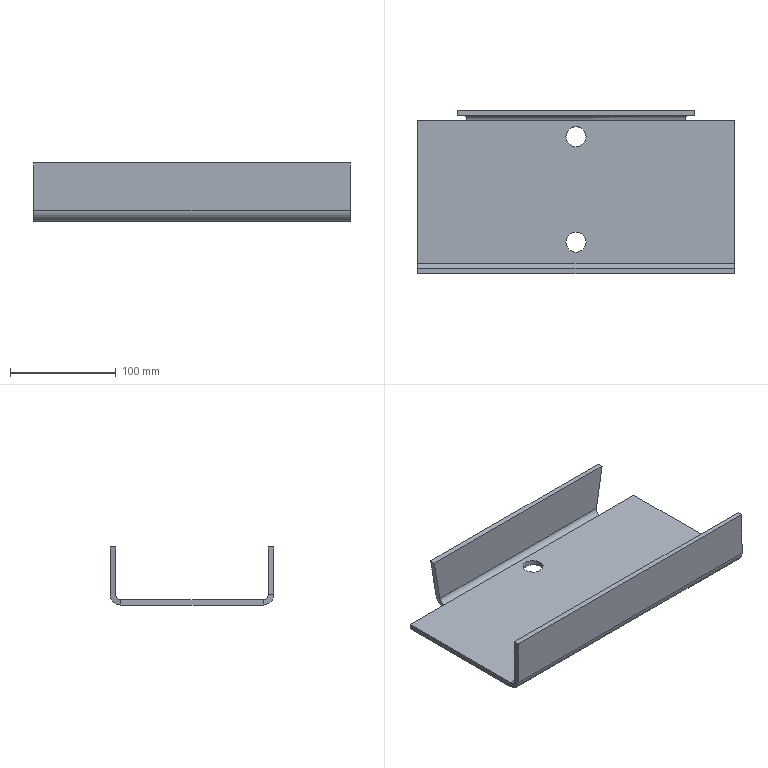Part | SolidWorks | features Split 2, FlatPattern 1, HoleWzd 1, SM3dBend 1, SMBaseFlange 1, SheetMetal 1 | 1 solid | 26 faces | box 300 x 155 x 54.999 mm | volume 345967 mm3 | plane 18 | cylinder 8 | commonest cylinder face diameters 19 x4 10 x2 20 x2
STEP:
#1=CARTESIAN_POINT('',(9.5,52.5,0.));
#2=VERTEX_POINT('',#1);
#3=CARTESIAN_POINT('',(-9.5,52.5,0.));
#4=VERTEX_POINT('',#3);
#5=CARTESIAN_POINT('',(0.,52.5,0.));
#6=DIRECTION('',(0.,0.,-1.));
#7=DIRECTION('',(1.,0.,0.));
#8=AXIS2_PLACEMENT_3D('',#5,#6,#7);
#9=CIRCLE('',#8,9.5);
#10=EDGE_CURVE('',#2,#4,#9,.T.);
#11=ORIENTED_EDGE('',*,*,#10,.F.);
#12=CARTESIAN_POINT('',(9.5,52.5,-5.));
#13=VERTEX_POINT('',#12);
#14=CARTESIAN_POINT('',(9.5,52.5,-5.));
#15=DIRECTION('',(0.,0.,-1.));
#16=VECTOR('',#15,1000.);
#17=LINE('',#14,#16);
#18=EDGE_CURVE('',#2,#13,#17,.T.);
#19=ORIENTED_EDGE('',*,*,#18,.T.);
#20=CARTESIAN_POINT('',(-9.5,52.5,-5.));
#21=VERTEX_POINT('',#20);
#22=CARTESIAN_POINT('',(0.,52.5,-5.));
#23=DIRECTION('',(0.,0.,-1.));
#24=DIRECTION('',(-1.,0.,0.));
#25=AXIS2_PLACEMENT_3D('',#22,#23,#24);
#26=CIRCLE('',#25,9.5);
#27=EDGE_CURVE('',#13,#21,#26,.T.);
#28=ORIENTED_EDGE('',*,*,#27,.T.);
#29=CARTESIAN_POINT('',(-9.5,52.5,-5.));
#30=DIRECTION('',(0.,0.,-1.));
#31=VECTOR('',#30,1000.);
#32=LINE('',#29,#31);
#33=EDGE_CURVE('',#4,#21,#32,.T.);
#34=ORIENTED_EDGE('',*,*,#33,.F.);
#35=EDGE_LOOP('',(#11,#19,#28,#34));
#36=FACE_OUTER_BOUND('',#35,.T.);
#37=CARTESIAN_POINT('',(0.,52.5,-5.));
#38=DIRECTION('',(0.,0.,-1.));
#39=DIRECTION('',(-1.,0.,0.));
#40=AXIS2_PLACEMENT_3D('',#37,#38,#39);
#41=CYLINDRICAL_SURFACE('',#40,9.5);
#42=ADVANCED_FACE('',(#36),#41,.F.);
#43=CARTESIAN_POINT('',(9.5,-47.5,0.));
#44=VERTEX_POINT('',#43);
#45=CARTESIAN_POINT('',(-9.5,-47.5,0.));
#46=VERTEX_POINT('',#45);
#47=CARTESIAN_POINT('',(0.,-47.5,0.));
#48=DIRECTION('',(0.,0.,-1.));
#49=DIRECTION('',(1.,0.,0.));
#50=AXIS2_PLACEMENT_3D('',#47,#48,#49);
#51=CIRCLE('',#50,9.5);
#52=EDGE_CURVE('',#44,#46,#51,.T.);
#53=ORIENTED_EDGE('',*,*,#52,.F.);
#54=CARTESIAN_POINT('',(9.5,-47.5,-5.));
#55=VERTEX_POINT('',#54);
#56=CARTESIAN_POINT('',(9.5,-47.5,-5.));
#57=DIRECTION('',(0.,0.,-1.));
#58=VECTOR('',#57,1000.);
#59=LINE('',#56,#58);
#60=EDGE_CURVE('',#44,#55,#59,.T.);
#61=ORIENTED_EDGE('',*,*,#60,.T.);
#62=CARTESIAN_POINT('',(-9.5,-47.5,-5.));
#63=VERTEX_POINT('',#62);
#64=CARTESIAN_POINT('',(0.,-47.5,-5.));
#65=DIRECTION('',(0.,0.,-1.));
#66=DIRECTION('',(-1.,0.,0.));
#67=AXIS2_PLACEMENT_3D('',#64,#65,#66);
#68=CIRCLE('',#67,9.5);
#69=EDGE_CURVE('',#55,#63,#68,.T.);
#70=ORIENTED_EDGE('',*,*,#69,.T.);
#71=CARTESIAN_POINT('',(-9.5,-47.5,-5.));
#72=DIRECTION('',(0.,0.,-1.));
#73=VECTOR('',#72,1000.);
#74=LINE('',#71,#73);
#75=EDGE_CURVE('',#46,#63,#74,.T.);
#76=ORIENTED_EDGE('',*,*,#75,.F.);
#77=EDGE_LOOP('',(#53,#61,#70,#76));
#78=FACE_OUTER_BOUND('',#77,.T.);
#79=CARTESIAN_POINT('',(0.,-47.5,-5.));
#80=DIRECTION('',(0.,0.,-1.));
#81=DIRECTION('',(-1.,0.,0.));
#82=AXIS2_PLACEMENT_3D('',#79,#80,#81);
#83=CYLINDRICAL_SURFACE('',#82,9.5);
#84=ADVANCED_FACE('',(#78),#83,.F.);
#85=CARTESIAN_POINT('',(103.165,67.5,-5.));
#86=VERTEX_POINT('',#85);
#87=CARTESIAN_POINT('',(104.001,67.5,0.));
#88=VERTEX_POINT('',#87);
#89=CARTESIAN_POINT('',(101.168,67.5,-16.93));
#90=DIRECTION('',(0.165,0.,0.9863));
#91=VECTOR('',#90,1000.);
#92=LINE('',#89,#91);
#93=EDGE_CURVE('',#86,#88,#92,.T.);
#94=ORIENTED_EDGE('',*,*,#93,.F.);
#95=CARTESIAN_POINT('',(104.838,77.5,5.));
#96=VERTEX_POINT('',#95);
#97=CARTESIAN_POINT('',(103.165,67.5,-5.));
#98=CARTESIAN_POINT('',(103.165,73.358,-5.));
#99=CARTESIAN_POINT('',(103.858,77.5,-0.8579));
#100=CARTESIAN_POINT('',(104.838,77.5,5.));
#101=(BOUNDED_CURVE()B_SPLINE_CURVE(3,(#97,#98,#99,#100),.UNSPECIFIED.,.F.,.F.)B_SPLINE_CURVE_WITH_KNOTS((4,4),(3.142,4.712),.UNSPECIFIED.)CURVE()GEOMETRIC_REPRESENTATION_ITEM()RATIONAL_B_SPLINE_CURVE((1.,0.8047,0.8047,1.))REPRESENTATION_ITEM(''));
#102=EDGE_CURVE('',#86,#96,#101,.T.);
#103=ORIENTED_EDGE('',*,*,#102,.T.);
#104=CARTESIAN_POINT('',(112.368,77.5,49.999));
#105=VERTEX_POINT('',#104);
#106=CARTESIAN_POINT('',(89.077,77.5,-89.187));
#107=DIRECTION('',(-0.165,0.,-0.9863));
#108=VECTOR('',#107,1000.);
#109=LINE('',#106,#108);
#110=EDGE_CURVE('',#105,#96,#109,.T.);
#111=ORIENTED_EDGE('',*,*,#110,.F.);
#112=CARTESIAN_POINT('',(112.368,72.5,49.999));
#113=VERTEX_POINT('',#112);
#114=CARTESIAN_POINT('',(112.368,77.5,49.999));
#115=DIRECTION('',(0.,-1.,0.));
#116=VECTOR('',#115,1000.);
#117=LINE('',#114,#116);
#118=EDGE_CURVE('',#105,#113,#117,.T.);
#119=ORIENTED_EDGE('',*,*,#118,.T.);
#120=CARTESIAN_POINT('',(104.838,72.5,5.));
#121=VERTEX_POINT('',#120);
#122=CARTESIAN_POINT('',(89.077,72.5,-89.187));
#123=DIRECTION('',(-0.165,0.,-0.9863));
#124=VECTOR('',#123,1000.);
#125=LINE('',#122,#124);
#126=EDGE_CURVE('',#113,#121,#125,.T.);
#127=ORIENTED_EDGE('',*,*,#126,.T.);
#128=CARTESIAN_POINT('',(104.001,67.5,0.));
#129=CARTESIAN_POINT('',(104.001,70.429,0.));
#130=CARTESIAN_POINT('',(104.348,72.5,2.071));
#131=CARTESIAN_POINT('',(104.838,72.5,5.));
#132=(BOUNDED_CURVE()B_SPLINE_CURVE(3,(#128,#129,#130,#131),.UNSPECIFIED.,.F.,.F.)B_SPLINE_CURVE_WITH_KNOTS((4,4),(3.142,4.712),.UNSPECIFIED.)CURVE()GEOMETRIC_REPRESENTATION_ITEM()RATIONAL_B_SPLINE_CURVE((1.,0.8047,0.8047,1.))REPRESENTATION_ITEM(''));
#133=EDGE_CURVE('',#88,#121,#132,.T.);
#134=ORIENTED_EDGE('',*,*,#133,.F.);
#135=EDGE_LOOP('',(#94,#103,#111,#119,#127,#134));
#136=FACE_OUTER_BOUND('',#135,.T.);
#137=CARTESIAN_POINT('',(101.168,0.,-16.93));
#138=DIRECTION('',(-0.9863,0.,0.165));
#139=DIRECTION('',(0.165,0.,0.9863));
#140=AXIS2_PLACEMENT_3D('',#137,#138,#139);
#141=PLANE('',#140);
#142=ADVANCED_FACE('',(#136),#141,.F.);
#143=CARTESIAN_POINT('',(-104.032,67.5,0.));
#144=VERTEX_POINT('',#143);
#145=CARTESIAN_POINT('',(-150.,67.5,0.));
#146=VERTEX_POINT('',#145);
#147=CARTESIAN_POINT('',(0.,67.5,0.));
#148=DIRECTION('',(-1.,0.,0.));
#149=VECTOR('',#148,1000.);
#150=LINE('',#147,#149);
#151=EDGE_CURVE('',#144,#146,#150,.T.);
#152=ORIENTED_EDGE('',*,*,#151,.F.);
#153=CARTESIAN_POINT('',(-103.195,67.5,-5.));
#154=VERTEX_POINT('',#153);
#155=CARTESIAN_POINT('',(-101.198,67.5,-16.935));
#156=DIRECTION('',(0.165,0.,-0.9863));
#157=VECTOR('',#156,1000.);
#158=LINE('',#155,#157);
#159=EDGE_CURVE('',#144,#154,#158,.T.);
#160=ORIENTED_EDGE('',*,*,#159,.T.);
#161=CARTESIAN_POINT('',(-150.,67.5,-5.));
#162=VERTEX_POINT('',#161);
#163=CARTESIAN_POINT('',(0.,67.5,-5.));
#164=DIRECTION('',(-1.,0.,0.));
#165=VECTOR('',#164,1000.);
#166=LINE('',#163,#165);
#167=EDGE_CURVE('',#154,#162,#166,.T.);
#168=ORIENTED_EDGE('',*,*,#167,.T.);
#169=CARTESIAN_POINT('',(-150.,67.5,-5.));
#170=DIRECTION('',(0.,0.,-1.));
#171=VECTOR('',#170,1000.);
#172=LINE('',#169,#171);
#173=EDGE_CURVE('',#146,#162,#172,.T.);
#174=ORIENTED_EDGE('',*,*,#173,.F.);
#175=EDGE_LOOP('',(#152,#160,#168,#174));
#176=FACE_OUTER_BOUND('',#175,.T.);
#177=CARTESIAN_POINT('',(0.,67.5,0.));
#178=DIRECTION('',(0.,1.,0.));
#179=DIRECTION('',(0.,0.,1.));
#180=AXIS2_PLACEMENT_3D('',#177,#178,#179);
#181=PLANE('',#180);
#182=ADVANCED_FACE('',(#176),#181,.T.);
#183=CARTESIAN_POINT('',(-150.,-72.5,49.999));
#184=VERTEX_POINT('',#183);
#185=CARTESIAN_POINT('',(150.,-72.5,49.999));
#186=VERTEX_POINT('',#185);
#187=CARTESIAN_POINT('',(-150.,-72.5,49.999));
#188=DIRECTION('',(1.,0.,0.));
#189=VECTOR('',#188,1000.);
#190=LINE('',#187,#189);
#191=EDGE_CURVE('',#184,#186,#190,.T.);
#192=ORIENTED_EDGE('',*,*,#191,.T.);
#193=CARTESIAN_POINT('',(150.,-72.5,5.));
#194=VERTEX_POINT('',#193);
#195=CARTESIAN_POINT('',(150.,-72.5,-198.561));
#196=DIRECTION('',(0.,0.,-1.));
#197=VECTOR('',#196,1000.);
#198=LINE('',#195,#197);
#199=EDGE_CURVE('',#186,#194,#198,.T.);
#200=ORIENTED_EDGE('',*,*,#199,.T.);
#201=CARTESIAN_POINT('',(-150.,-72.5,5.));
#202=VERTEX_POINT('',#201);
#203=CARTESIAN_POINT('',(0.,-72.5,5.));
#204=DIRECTION('',(-1.,0.,0.));
#205=VECTOR('',#204,1000.);
#206=LINE('',#203,#205);
#207=EDGE_CURVE('',#194,#202,#206,.T.);
#208=ORIENTED_EDGE('',*,*,#207,.T.);
#209=CARTESIAN_POINT('',(-150.,-72.5,-198.561));
#210=DIRECTION('',(0.,0.,1.));
#211=VECTOR('',#210,1000.);
#212=LINE('',#209,#211);
#213=EDGE_CURVE('',#202,#184,#212,.T.);
#214=ORIENTED_EDGE('',*,*,#213,.T.);
#215=EDGE_LOOP('',(#192,#200,#208,#214));
#216=FACE_OUTER_BOUND('',#215,.T.);
#217=CARTESIAN_POINT('',(0.,-72.5,-74.281));
#218=DIRECTION('',(0.,1.,0.));
#219=DIRECTION('',(1.,0.,0.));
#220=AXIS2_PLACEMENT_3D('',#217,#218,#219);
#221=PLANE('',#220);
#222=ADVANCED_FACE('',(#216),#221,.T.);
#223=ORIENTED_EDGE('',*,*,#207,.F.);
#224=CARTESIAN_POINT('',(150.,-67.5,0.));
#225=VERTEX_POINT('',#224);
#226=CARTESIAN_POINT('',(150.,-67.5,5.));
#227=DIRECTION('',(-1.,0.,0.));
#228=DIRECTION('',(0.,0.,1.));
#229=AXIS2_PLACEMENT_3D('',#226,#227,#228);
#230=CIRCLE('',#229,5.);
#231=EDGE_CURVE('',#225,#194,#230,.T.);
#232=ORIENTED_EDGE('',*,*,#231,.F.);
#233=CARTESIAN_POINT('',(-150.,-67.5,0.));
#234=VERTEX_POINT('',#233);
#235=CARTESIAN_POINT('',(0.,-67.5,0.));
#236=DIRECTION('',(-1.,0.,0.));
#237=VECTOR('',#236,1000.);
#238=LINE('',#235,#237);
#239=EDGE_CURVE('',#225,#234,#238,.T.);
#240=ORIENTED_EDGE('',*,*,#239,.T.);
#241=CARTESIAN_POINT('',(-150.,-67.5,5.));
#242=DIRECTION('',(1.,0.,0.));
#243=DIRECTION('',(0.,0.,1.));
#244=AXIS2_PLACEMENT_3D('',#241,#242,#243);
#245=CIRCLE('',#244,5.);
#246=EDGE_CURVE('',#202,#234,#245,.T.);
#247=ORIENTED_EDGE('',*,*,#246,.F.);
#248=EDGE_LOOP('',(#223,#232,#240,#247));
#249=FACE_OUTER_BOUND('',#248,.T.);
#250=CARTESIAN_POINT('',(300.273,-67.5,5.));
#251=DIRECTION('',(-1.,0.,0.));
#252=DIRECTION('',(0.,0.,1.));
#253=AXIS2_PLACEMENT_3D('',#250,#251,#252);
#254=CYLINDRICAL_SURFACE('',#253,5.);
#255=ADVANCED_FACE('',(#249),#254,.F.);
#256=CARTESIAN_POINT('',(150.,-77.5,5.));
#257=VERTEX_POINT('',#256);
#258=CARTESIAN_POINT('',(-150.,-77.5,5.));
#259=VERTEX_POINT('',#258);
#260=CARTESIAN_POINT('',(0.,-77.5,5.));
#261=DIRECTION('',(-1.,0.,0.));
#262=VECTOR('',#261,1000.);
#263=LINE('',#260,#262);
#264=EDGE_CURVE('',#257,#259,#263,.T.);
#265=ORIENTED_EDGE('',*,*,#264,.F.);
#266=CARTESIAN_POINT('',(150.,-77.5,49.999));
#267=VERTEX_POINT('',#266);
#268=CARTESIAN_POINT('',(150.,-77.5,-198.561));
#269=DIRECTION('',(0.,0.,-1.));
#270=VECTOR('',#269,1000.);
#271=LINE('',#268,#270);
#272=EDGE_CURVE('',#267,#257,#271,.T.);
#273=ORIENTED_EDGE('',*,*,#272,.F.);
#274=CARTESIAN_POINT('',(-150.,-77.5,49.999));
#275=VERTEX_POINT('',#274);
#276=CARTESIAN_POINT('',(-150.,-77.5,49.999));
#277=DIRECTION('',(1.,0.,0.));
#278=VECTOR('',#277,1000.);
#279=LINE('',#276,#278);
#280=EDGE_CURVE('',#275,#267,#279,.T.);
#281=ORIENTED_EDGE('',*,*,#280,.F.);
#282=CARTESIAN_POINT('',(-150.,-77.5,-198.561));
#283=DIRECTION('',(0.,0.,1.));
#284=VECTOR('',#283,1000.);
#285=LINE('',#282,#284);
#286=EDGE_CURVE('',#259,#275,#285,.T.);
#287=ORIENTED_EDGE('',*,*,#286,.F.);
#288=EDGE_LOOP('',(#265,#273,#281,#287));
#289=FACE_OUTER_BOUND('',#288,.T.);
#290=CARTESIAN_POINT('',(0.,-77.5,-74.281));
#291=DIRECTION('',(0.,1.,0.));
#292=DIRECTION('',(1.,0.,0.));
#293=AXIS2_PLACEMENT_3D('',#290,#291,#292);
#294=PLANE('',#293);
#295=ADVANCED_FACE('',(#289),#294,.F.);
#296=CARTESIAN_POINT('',(150.,-67.5,-5.));
#297=VERTEX_POINT('',#296);
#298=CARTESIAN_POINT('',(-150.,-67.5,-5.));
#299=VERTEX_POINT('',#298);
#300=CARTESIAN_POINT('',(0.,-67.5,-5.));
#301=DIRECTION('',(-1.,0.,0.));
#302=VECTOR('',#301,1000.);
#303=LINE('',#300,#302);
#304=EDGE_CURVE('',#297,#299,#303,.T.);
#305=ORIENTED_EDGE('',*,*,#304,.F.);
#306=CARTESIAN_POINT('',(150.,-67.5,5.));
#307=DIRECTION('',(-1.,0.,0.));
#308=DIRECTION('',(0.,0.,-1.));
#309=AXIS2_PLACEMENT_3D('',#306,#307,#308);
#310=CIRCLE('',#309,10.);
#311=EDGE_CURVE('',#297,#257,#310,.T.);
#312=ORIENTED_EDGE('',*,*,#311,.T.);
#313=ORIENTED_EDGE('',*,*,#264,.T.);
#314=CARTESIAN_POINT('',(-150.,-67.5,5.));
#315=DIRECTION('',(1.,0.,0.));
#316=DIRECTION('',(0.,0.,1.));
#317=AXIS2_PLACEMENT_3D('',#314,#315,#316);
#318=CIRCLE('',#317,10.);
#319=EDGE_CURVE('',#259,#299,#318,.T.);
#320=ORIENTED_EDGE('',*,*,#319,.T.);
#321=EDGE_LOOP('',(#305,#312,#313,#320));
#322=FACE_OUTER_BOUND('',#321,.T.);
#323=CARTESIAN_POINT('',(300.273,-67.5,5.));
#324=DIRECTION('',(-1.,0.,0.));
#325=DIRECTION('',(0.,0.,1.));
#326=AXIS2_PLACEMENT_3D('',#323,#324,#325);
#327=CYLINDRICAL_SURFACE('',#326,10.);
#328=ADVANCED_FACE('',(#322),#327,.T.);
#329=ORIENTED_EDGE('',*,*,#280,.T.);
#330=CARTESIAN_POINT('',(150.,-77.5,49.999));
#331=DIRECTION('',(0.,1.,0.));
#332=VECTOR('',#331,1000.);
#333=LINE('',#330,#332);
#334=EDGE_CURVE('',#267,#186,#333,.T.);
#335=ORIENTED_EDGE('',*,*,#334,.T.);
#336=ORIENTED_EDGE('',*,*,#191,.F.);
#337=CARTESIAN_POINT('',(-150.,-77.5,49.999));
#338=DIRECTION('',(0.,1.,0.));
#339=VECTOR('',#338,1000.);
#340=LINE('',#337,#339);
#341=EDGE_CURVE('',#275,#184,#340,.T.);
#342=ORIENTED_EDGE('',*,*,#341,.F.);
#343=EDGE_LOOP('',(#329,#335,#336,#342));
#344=FACE_OUTER_BOUND('',#343,.T.);
#345=CARTESIAN_POINT('',(-150.,-77.5,49.999));
#346=DIRECTION('',(0.,0.,1.));
#347=DIRECTION('',(0.,-1.,0.));
#348=AXIS2_PLACEMENT_3D('',#345,#346,#347);
#349=PLANE('',#348);
#350=ADVANCED_FACE('',(#344),#349,.T.);
#351=ORIENTED_EDGE('',*,*,#213,.F.);
#352=CARTESIAN_POINT('',(-150.,-77.5,5.));
#353=DIRECTION('',(0.,-1.,0.));
#354=VECTOR('',#353,1000.);
#355=LINE('',#352,#354);
#356=EDGE_CURVE('',#202,#259,#355,.T.);
#357=ORIENTED_EDGE('',*,*,#356,.T.);
#358=ORIENTED_EDGE('',*,*,#286,.T.);
#359=ORIENTED_EDGE('',*,*,#341,.T.);
#360=EDGE_LOOP('',(#351,#357,#358,#359));
#361=FACE_OUTER_BOUND('',#360,.T.);
#362=CARTESIAN_POINT('',(-150.,-77.5,-198.561));
#363=DIRECTION('',(-1.,0.,0.));
#364=DIRECTION('',(0.,0.,1.));
#365=AXIS2_PLACEMENT_3D('',#362,#363,#364);
#366=PLANE('',#365);
#367=ADVANCED_FACE('',(#361),#366,.T.);
#368=CARTESIAN_POINT('',(-150.,-67.5,-5.));
#369=DIRECTION('',(0.,0.,-1.));
#370=VECTOR('',#369,1000.);
#371=LINE('',#368,#370);
#372=EDGE_CURVE('',#234,#299,#371,.T.);
#373=ORIENTED_EDGE('',*,*,#372,.F.);
#374=CARTESIAN_POINT('',(-150.,124.28,0.));
#375=DIRECTION('',(0.,-1.,0.));
#376=VECTOR('',#375,1000.);
#377=LINE('',#374,#376);
#378=EDGE_CURVE('',#146,#234,#377,.T.);
#379=ORIENTED_EDGE('',*,*,#378,.F.);
#380=ORIENTED_EDGE('',*,*,#173,.T.);
#381=CARTESIAN_POINT('',(-150.,124.28,-5.));
#382=DIRECTION('',(0.,-1.,0.));
#383=VECTOR('',#382,1000.);
#384=LINE('',#381,#383);
#385=EDGE_CURVE('',#162,#299,#384,.T.);
#386=ORIENTED_EDGE('',*,*,#385,.T.);
#387=EDGE_LOOP('',(#373,#379,#380,#386));
#388=FACE_OUTER_BOUND('',#387,.T.);
#389=CARTESIAN_POINT('',(-150.,124.28,-5.));
#390=DIRECTION('',(-1.,0.,0.));
#391=DIRECTION('',(0.,-1.,0.));
#392=AXIS2_PLACEMENT_3D('',#389,#390,#391);
#393=PLANE('',#392);
#394=ADVANCED_FACE('',(#388),#393,.T.);
#395=ORIENTED_EDGE('',*,*,#356,.F.);
#396=ORIENTED_EDGE('',*,*,#246,.T.);
#397=ORIENTED_EDGE('',*,*,#372,.T.);
#398=ORIENTED_EDGE('',*,*,#319,.F.);
#399=EDGE_LOOP('',(#395,#396,#397,#398));
#400=FACE_OUTER_BOUND('',#399,.T.);
#401=CARTESIAN_POINT('',(-150.,-67.5,5.));
#402=DIRECTION('',(-1.,0.,0.));
#403=DIRECTION('',(0.,0.,1.));
#404=AXIS2_PLACEMENT_3D('',#401,#402,#403);
#405=PLANE('',#404);
#406=ADVANCED_FACE('',(#400),#405,.T.);
#407=CARTESIAN_POINT('',(0.,52.5,0.));
#408=DIRECTION('',(0.,0.,-1.));
#409=DIRECTION('',(1.,0.,0.));
#410=AXIS2_PLACEMENT_3D('',#407,#408,#409);
#411=CIRCLE('',#410,9.5);
#412=EDGE_CURVE('',#4,#2,#411,.T.);
#413=ORIENTED_EDGE('',*,*,#412,.T.);
#414=ORIENTED_EDGE('',*,*,#10,.T.);
#415=EDGE_LOOP('',(#413,#414));
#416=FACE_BOUND('',#415,.T.);
#417=CARTESIAN_POINT('',(0.,-47.5,0.));
#418=DIRECTION('',(0.,0.,-1.));
#419=DIRECTION('',(1.,0.,0.));
#420=AXIS2_PLACEMENT_3D('',#417,#418,#419);
#421=CIRCLE('',#420,9.5);
#422=EDGE_CURVE('',#46,#44,#421,.T.);
#423=ORIENTED_EDGE('',*,*,#422,.T.);
#424=ORIENTED_EDGE('',*,*,#52,.T.);
#425=EDGE_LOOP('',(#423,#424));
#426=FACE_BOUND('',#425,.T.);
#427=ORIENTED_EDGE('',*,*,#239,.F.);
#428=CARTESIAN_POINT('',(150.,67.5,0.));
#429=VERTEX_POINT('',#428);
#430=CARTESIAN_POINT('',(150.,124.28,0.));
#431=DIRECTION('',(0.,1.,0.));
#432=VECTOR('',#431,1000.);
#433=LINE('',#430,#432);
#434=EDGE_CURVE('',#225,#429,#433,.T.);
#435=ORIENTED_EDGE('',*,*,#434,.T.);
#436=CARTESIAN_POINT('',(0.,67.5,0.));
#437=DIRECTION('',(-1.,0.,0.));
#438=VECTOR('',#437,1000.);
#439=LINE('',#436,#438);
#440=EDGE_CURVE('',#429,#88,#439,.T.);
#441=ORIENTED_EDGE('',*,*,#440,.T.);
#442=CARTESIAN_POINT('',(0.,67.5,0.));
#443=DIRECTION('',(-1.,0.,0.));
#444=VECTOR('',#443,1000.);
#445=LINE('',#442,#444);
#446=EDGE_CURVE('',#88,#144,#445,.T.);
#447=ORIENTED_EDGE('',*,*,#446,.T.);
#448=ORIENTED_EDGE('',*,*,#151,.T.);
#449=ORIENTED_EDGE('',*,*,#378,.T.);
#450=EDGE_LOOP('',(#427,#435,#441,#447,#448,#449));
#451=FACE_OUTER_BOUND('',#450,.T.);
#452=CARTESIAN_POINT('',(0.,0.,0.));
#453=DIRECTION('',(0.,0.,1.));
#454=DIRECTION('',(1.,0.,0.));
#455=AXIS2_PLACEMENT_3D('',#452,#453,#454);
#456=PLANE('',#455);
#457=ADVANCED_FACE('',(#416,#426,#451),#456,.T.);
#458=CARTESIAN_POINT('',(0.,52.5,-5.));
#459=DIRECTION('',(0.,0.,-1.));
#460=DIRECTION('',(-1.,0.,0.));
#461=AXIS2_PLACEMENT_3D('',#458,#459,#460);
#462=CIRCLE('',#461,9.5);
#463=EDGE_CURVE('',#21,#13,#462,.T.);
#464=ORIENTED_EDGE('',*,*,#463,.F.);
#465=ORIENTED_EDGE('',*,*,#27,.F.);
#466=EDGE_LOOP('',(#464,#465));
#467=FACE_BOUND('',#466,.T.);
#468=CARTESIAN_POINT('',(0.,-47.5,-5.));
#469=DIRECTION('',(0.,0.,-1.));
#470=DIRECTION('',(-1.,0.,0.));
#471=AXIS2_PLACEMENT_3D('',#468,#469,#470);
#472=CIRCLE('',#471,9.5);
#473=EDGE_CURVE('',#63,#55,#472,.T.);
#474=ORIENTED_EDGE('',*,*,#473,.F.);
#475=ORIENTED_EDGE('',*,*,#69,.F.);
#476=EDGE_LOOP('',(#474,#475));
#477=FACE_BOUND('',#476,.T.);
#478=CARTESIAN_POINT('',(0.,67.5,-5.));
#479=DIRECTION('',(-1.,0.,0.));
#480=VECTOR('',#479,1000.);
#481=LINE('',#478,#480);
#482=EDGE_CURVE('',#86,#154,#481,.T.);
#483=ORIENTED_EDGE('',*,*,#482,.F.);
#484=CARTESIAN_POINT('',(150.,67.5,-5.));
#485=VERTEX_POINT('',#484);
#486=CARTESIAN_POINT('',(0.,67.5,-5.));
#487=DIRECTION('',(-1.,0.,0.));
#488=VECTOR('',#487,1000.);
#489=LINE('',#486,#488);
#490=EDGE_CURVE('',#485,#86,#489,.T.);
#491=ORIENTED_EDGE('',*,*,#490,.F.);
#492=CARTESIAN_POINT('',(150.,124.28,-5.));
#493=DIRECTION('',(0.,1.,0.));
#494=VECTOR('',#493,1000.);
#495=LINE('',#492,#494);
#496=EDGE_CURVE('',#297,#485,#495,.T.);
#497=ORIENTED_EDGE('',*,*,#496,.F.);
#498=ORIENTED_EDGE('',*,*,#304,.T.);
#499=ORIENTED_EDGE('',*,*,#385,.F.);
#500=ORIENTED_EDGE('',*,*,#167,.F.);
#501=EDGE_LOOP('',(#483,#491,#497,#498,#499,#500));
#502=FACE_OUTER_BOUND('',#501,.T.);
#503=CARTESIAN_POINT('',(0.,0.,-5.));
#504=DIRECTION('',(0.,0.,1.));
#505=DIRECTION('',(1.,0.,0.));
#506=AXIS2_PLACEMENT_3D('',#503,#504,#505);
#507=PLANE('',#506);
#508=ADVANCED_FACE('',(#467,#477,#502),#507,.F.);
#509=ORIENTED_EDGE('',*,*,#102,.F.);
#510=ORIENTED_EDGE('',*,*,#482,.T.);
#511=CARTESIAN_POINT('',(-104.868,77.5,5.));
#512=VERTEX_POINT('',#511);
#513=CARTESIAN_POINT('',(-104.868,77.5,5.));
#514=CARTESIAN_POINT('',(-103.888,77.5,-0.8579));
#515=CARTESIAN_POINT('',(-103.195,73.358,-5.));
#516=CARTESIAN_POINT('',(-103.195,67.5,-5.));
#517=(BOUNDED_CURVE()B_SPLINE_CURVE(3,(#513,#514,#515,#516),.UNSPECIFIED.,.F.,.F.)B_SPLINE_CURVE_WITH_KNOTS((4,4),(4.712,6.283),.UNSPECIFIED.)CURVE()GEOMETRIC_REPRESENTATION_ITEM()RATIONAL_B_SPLINE_CURVE((1.,0.8047,0.8047,1.))REPRESENTATION_ITEM(''));
#518=EDGE_CURVE('',#512,#154,#517,.T.);
#519=ORIENTED_EDGE('',*,*,#518,.F.);
#520=CARTESIAN_POINT('',(0.,77.5,5.));
#521=DIRECTION('',(-1.,0.,0.));
#522=VECTOR('',#521,1000.);
#523=LINE('',#520,#522);
#524=EDGE_CURVE('',#96,#512,#523,.T.);
#525=ORIENTED_EDGE('',*,*,#524,.F.);
#526=EDGE_LOOP('',(#509,#510,#519,#525));
#527=FACE_OUTER_BOUND('',#526,.T.);
#528=CARTESIAN_POINT('',(-300.273,67.5,5.));
#529=DIRECTION('',(1.,0.,0.));
#530=DIRECTION('',(0.,0.,-1.));
#531=AXIS2_PLACEMENT_3D('',#528,#529,#530);
#532=CYLINDRICAL_SURFACE('',#531,10.);
#533=ADVANCED_FACE('',(#527),#532,.T.);
#534=ORIENTED_EDGE('',*,*,#446,.F.);
#535=ORIENTED_EDGE('',*,*,#133,.T.);
#536=CARTESIAN_POINT('',(-104.868,72.5,5.));
#537=VERTEX_POINT('',#536);
#538=CARTESIAN_POINT('',(0.,72.5,5.));
#539=DIRECTION('',(-1.,0.,0.));
#540=VECTOR('',#539,1000.);
#541=LINE('',#538,#540);
#542=EDGE_CURVE('',#121,#537,#541,.T.);
#543=ORIENTED_EDGE('',*,*,#542,.T.);
#544=CARTESIAN_POINT('',(-104.868,72.5,5.));
#545=CARTESIAN_POINT('',(-104.378,72.5,2.071));
#546=CARTESIAN_POINT('',(-104.032,70.429,0.));
#547=CARTESIAN_POINT('',(-104.032,67.5,0.));
#548=(BOUNDED_CURVE()B_SPLINE_CURVE(3,(#544,#545,#546,#547),.UNSPECIFIED.,.F.,.F.)B_SPLINE_CURVE_WITH_KNOTS((4,4),(4.712,6.283),.UNSPECIFIED.)CURVE()GEOMETRIC_REPRESENTATION_ITEM()RATIONAL_B_SPLINE_CURVE((1.,0.8047,0.8047,1.))REPRESENTATION_ITEM(''));
#549=EDGE_CURVE('',#537,#144,#548,.T.);
#550=ORIENTED_EDGE('',*,*,#549,.T.);
#551=EDGE_LOOP('',(#534,#535,#543,#550));
#552=FACE_OUTER_BOUND('',#551,.T.);
#553=CARTESIAN_POINT('',(-300.273,67.5,5.));
#554=DIRECTION('',(1.,0.,0.));
#555=DIRECTION('',(0.,0.,-1.));
#556=AXIS2_PLACEMENT_3D('',#553,#554,#555);
#557=CYLINDRICAL_SURFACE('',#556,5.);
#558=ADVANCED_FACE('',(#552),#557,.F.);
#559=ORIENTED_EDGE('',*,*,#118,.F.);
#560=CARTESIAN_POINT('',(-112.398,77.5,49.999));
#561=VERTEX_POINT('',#560);
#562=CARTESIAN_POINT('',(-150.,77.5,49.999));
#563=DIRECTION('',(-1.,0.,0.));
#564=VECTOR('',#563,1000.);
#565=LINE('',#562,#564);
#566=EDGE_CURVE('',#105,#561,#565,.T.);
#567=ORIENTED_EDGE('',*,*,#566,.T.);
#568=CARTESIAN_POINT('',(-112.398,72.5,49.999));
#569=VERTEX_POINT('',#568);
#570=CARTESIAN_POINT('',(-112.398,77.5,49.999));
#571=DIRECTION('',(0.,1.,0.));
#572=VECTOR('',#571,1000.);
#573=LINE('',#570,#572);
#574=EDGE_CURVE('',#569,#561,#573,.T.);
#575=ORIENTED_EDGE('',*,*,#574,.F.);
#576=CARTESIAN_POINT('',(-150.,72.5,49.999));
#577=DIRECTION('',(-1.,0.,0.));
#578=VECTOR('',#577,1000.);
#579=LINE('',#576,#578);
#580=EDGE_CURVE('',#113,#569,#579,.T.);
#581=ORIENTED_EDGE('',*,*,#580,.F.);
#582=EDGE_LOOP('',(#559,#567,#575,#581));
#583=FACE_OUTER_BOUND('',#582,.T.);
#584=CARTESIAN_POINT('',(-150.,77.5,49.999));
#585=DIRECTION('',(0.,0.,1.));
#586=DIRECTION('',(0.,-1.,0.));
#587=AXIS2_PLACEMENT_3D('',#584,#585,#586);
#588=PLANE('',#587);
#589=ADVANCED_FACE('',(#583),#588,.T.);
#590=ORIENTED_EDGE('',*,*,#566,.F.);
#591=ORIENTED_EDGE('',*,*,#110,.T.);
#592=ORIENTED_EDGE('',*,*,#524,.T.);
#593=CARTESIAN_POINT('',(-89.106,77.5,-89.192));
#594=DIRECTION('',(-0.165,0.,0.9863));
#595=VECTOR('',#594,1000.);
#596=LINE('',#593,#595);
#597=EDGE_CURVE('',#512,#561,#596,.T.);
#598=ORIENTED_EDGE('',*,*,#597,.T.);
#599=EDGE_LOOP('',(#590,#591,#592,#598));
#600=FACE_OUTER_BOUND('',#599,.T.);
#601=CARTESIAN_POINT('',(0.,77.5,-74.281));
#602=DIRECTION('',(0.,-1.,0.));
#603=DIRECTION('',(1.,0.,0.));
#604=AXIS2_PLACEMENT_3D('',#601,#602,#603);
#605=PLANE('',#604);
#606=ADVANCED_FACE('',(#600),#605,.F.);
#607=ORIENTED_EDGE('',*,*,#126,.F.);
#608=ORIENTED_EDGE('',*,*,#580,.T.);
#609=CARTESIAN_POINT('',(-89.106,72.5,-89.192));
#610=DIRECTION('',(-0.165,0.,0.9863));
#611=VECTOR('',#610,1000.);
#612=LINE('',#609,#611);
#613=EDGE_CURVE('',#537,#569,#612,.T.);
#614=ORIENTED_EDGE('',*,*,#613,.F.);
#615=ORIENTED_EDGE('',*,*,#542,.F.);
#616=EDGE_LOOP('',(#607,#608,#614,#615));
#617=FACE_OUTER_BOUND('',#616,.T.);
#618=CARTESIAN_POINT('',(0.,72.5,-74.281));
#619=DIRECTION('',(0.,-1.,0.));
#620=DIRECTION('',(1.,0.,0.));
#621=AXIS2_PLACEMENT_3D('',#618,#619,#620);
#622=PLANE('',#621);
#623=ADVANCED_FACE('',(#617),#622,.T.);
#624=ORIENTED_EDGE('',*,*,#518,.T.);
#625=ORIENTED_EDGE('',*,*,#159,.F.);
#626=ORIENTED_EDGE('',*,*,#549,.F.);
#627=ORIENTED_EDGE('',*,*,#613,.T.);
#628=ORIENTED_EDGE('',*,*,#574,.T.);
#629=ORIENTED_EDGE('',*,*,#597,.F.);
#630=EDGE_LOOP('',(#624,#625,#626,#627,#628,#629));
#631=FACE_OUTER_BOUND('',#630,.T.);
#632=CARTESIAN_POINT('',(-101.198,0.,-16.935));
#633=DIRECTION('',(0.9863,0.,0.165));
#634=DIRECTION('',(0.165,0.,-0.9863));
#635=AXIS2_PLACEMENT_3D('',#632,#633,#634);
#636=PLANE('',#635);
#637=ADVANCED_FACE('',(#631),#636,.F.);
#638=ORIENTED_EDGE('',*,*,#496,.T.);
#639=CARTESIAN_POINT('',(150.,67.5,5.));
#640=DIRECTION('',(0.,0.,1.));
#641=VECTOR('',#640,1000.);
#642=LINE('',#639,#641);
#643=EDGE_CURVE('',#485,#429,#642,.T.);
#644=ORIENTED_EDGE('',*,*,#643,.T.);
#645=ORIENTED_EDGE('',*,*,#434,.F.);
#646=CARTESIAN_POINT('',(150.,-67.5,-5.));
#647=DIRECTION('',(0.,0.,1.));
#648=VECTOR('',#647,1000.);
#649=LINE('',#646,#648);
#650=EDGE_CURVE('',#297,#225,#649,.T.);
#651=ORIENTED_EDGE('',*,*,#650,.F.);
#652=EDGE_LOOP('',(#638,#644,#645,#651));
#653=FACE_OUTER_BOUND('',#652,.T.);
#654=CARTESIAN_POINT('',(150.,67.5,5.));
#655=DIRECTION('',(1.,0.,0.));
#656=DIRECTION('',(0.,0.,-1.));
#657=AXIS2_PLACEMENT_3D('',#654,#655,#656);
#658=PLANE('',#657);
#659=ADVANCED_FACE('',(#653),#658,.T.);
#660=ORIENTED_EDGE('',*,*,#650,.T.);
#661=ORIENTED_EDGE('',*,*,#231,.T.);
#662=CARTESIAN_POINT('',(150.,-77.5,5.));
#663=DIRECTION('',(0.,1.,0.));
#664=VECTOR('',#663,1000.);
#665=LINE('',#662,#664);
#666=EDGE_CURVE('',#257,#194,#665,.T.);
#667=ORIENTED_EDGE('',*,*,#666,.F.);
#668=ORIENTED_EDGE('',*,*,#311,.F.);
#669=EDGE_LOOP('',(#660,#661,#667,#668));
#670=FACE_OUTER_BOUND('',#669,.T.);
#671=CARTESIAN_POINT('',(150.,-67.5,5.));
#672=DIRECTION('',(1.,0.,0.));
#673=DIRECTION('',(0.,0.,-1.));
#674=AXIS2_PLACEMENT_3D('',#671,#672,#673);
#675=PLANE('',#674);
#676=ADVANCED_FACE('',(#670),#675,.T.);
#677=ORIENTED_EDGE('',*,*,#272,.T.);
#678=ORIENTED_EDGE('',*,*,#666,.T.);
#679=ORIENTED_EDGE('',*,*,#199,.F.);
#680=ORIENTED_EDGE('',*,*,#334,.F.);
#681=EDGE_LOOP('',(#677,#678,#679,#680));
#682=FACE_OUTER_BOUND('',#681,.T.);
#683=CARTESIAN_POINT('',(150.,-77.5,-198.561));
#684=DIRECTION('',(1.,0.,0.));
#685=DIRECTION('',(0.,-1.,0.));
#686=AXIS2_PLACEMENT_3D('',#683,#684,#685);
#687=PLANE('',#686);
#688=ADVANCED_FACE('',(#682),#687,.T.);
#689=ORIENTED_EDGE('',*,*,#643,.F.);
#690=ORIENTED_EDGE('',*,*,#490,.T.);
#691=ORIENTED_EDGE('',*,*,#93,.T.);
#692=ORIENTED_EDGE('',*,*,#440,.F.);
#693=EDGE_LOOP('',(#689,#690,#691,#692));
#694=FACE_OUTER_BOUND('',#693,.T.);
#695=CARTESIAN_POINT('',(0.,67.5,0.));
#696=DIRECTION('',(0.,1.,0.));
#697=DIRECTION('',(0.,0.,1.));
#698=AXIS2_PLACEMENT_3D('',#695,#696,#697);
#699=PLANE('',#698);
#700=ADVANCED_FACE('',(#694),#699,.T.);
#701=ORIENTED_EDGE('',*,*,#60,.F.);
#702=ORIENTED_EDGE('',*,*,#422,.F.);
#703=ORIENTED_EDGE('',*,*,#75,.T.);
#704=ORIENTED_EDGE('',*,*,#473,.T.);
#705=EDGE_LOOP('',(#701,#702,#703,#704));
#706=FACE_OUTER_BOUND('',#705,.T.);
#707=CARTESIAN_POINT('',(0.,-47.5,-5.));
#708=DIRECTION('',(0.,0.,-1.));
#709=DIRECTION('',(-1.,0.,0.));
#710=AXIS2_PLACEMENT_3D('',#707,#708,#709);
#711=CYLINDRICAL_SURFACE('',#710,9.5);
#712=ADVANCED_FACE('',(#706),#711,.F.);
#713=ORIENTED_EDGE('',*,*,#18,.F.);
#714=ORIENTED_EDGE('',*,*,#412,.F.);
#715=ORIENTED_EDGE('',*,*,#33,.T.);
#716=ORIENTED_EDGE('',*,*,#463,.T.);
#717=EDGE_LOOP('',(#713,#714,#715,#716));
#718=FACE_OUTER_BOUND('',#717,.T.);
#719=CARTESIAN_POINT('',(0.,52.5,-5.));
#720=DIRECTION('',(0.,0.,-1.));
#721=DIRECTION('',(-1.,0.,0.));
#722=AXIS2_PLACEMENT_3D('',#719,#720,#721);
#723=CYLINDRICAL_SURFACE('',#722,9.5);
#724=ADVANCED_FACE('',(#718),#723,.F.);
#725=CLOSED_SHELL('',(#42,#84,#142,#182,#222,#255,#295,#328,#350,#367,#394,#406,#457,#508,#533,#558,#589,#606,#623,#637,#659,#676,#688,#700,#712,#724));
#726=MANIFOLD_SOLID_BREP('',#725);
#727=CARTESIAN_POINT('',(0.,0.,0.));
#728=DIRECTION('',(0.,0.,1.));
#729=DIRECTION('',(1.,0.,0.));
#730=AXIS2_PLACEMENT_3D('',#727,#728,#729);
#731=(LENGTH_UNIT()NAMED_UNIT(*)SI_UNIT(.MILLI.,.METRE.));
#732=UNCERTAINTY_MEASURE_WITH_UNIT(LENGTH_MEASURE(0.00001),#731,'','');
#733=(NAMED_UNIT(*)PLANE_ANGLE_UNIT()SI_UNIT($,.RADIAN.));
#734=(NAMED_UNIT(*)SI_UNIT($,.STERADIAN.)SOLID_ANGLE_UNIT());
#735=(GEOMETRIC_REPRESENTATION_CONTEXT(3)GLOBAL_UNCERTAINTY_ASSIGNED_CONTEXT((#732))GLOBAL_UNIT_ASSIGNED_CONTEXT((#731,#733,#734))REPRESENTATION_CONTEXT('',''));
#736=ADVANCED_BREP_SHAPE_REPRESENTATION('',(#726,#730),#735);